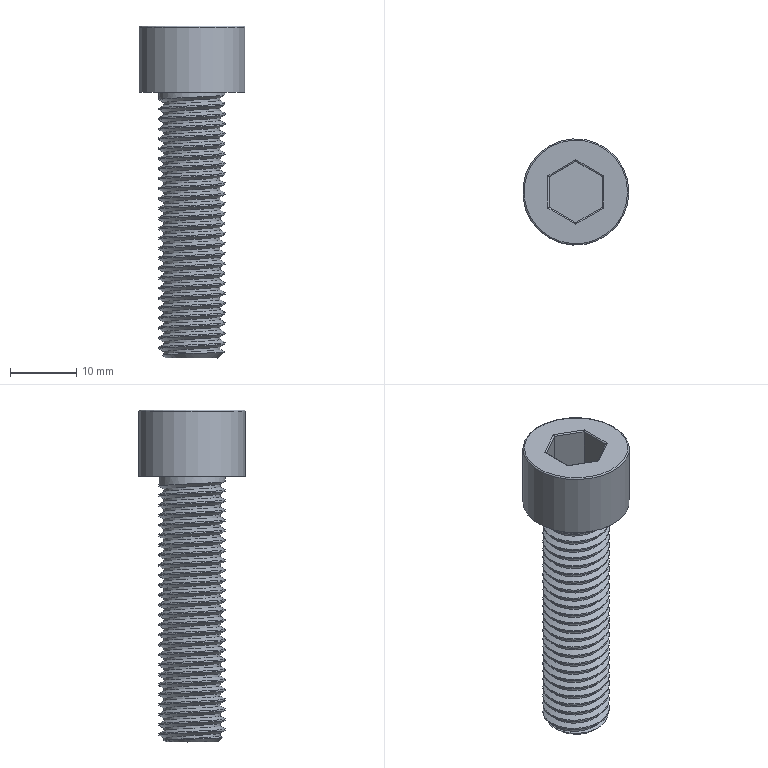Part | STEP file | Tube feed_id1718_x_t | 1 solid | 26 faces | box 16 x 16 x 50 mm | volume 4397 mm3 | plane 11 | cylinder 9 | spline 3 | cone 2 | torus 1 | commonest cylinder face diameters 0.4 x6 8.5 x1 10 x1 16 x1